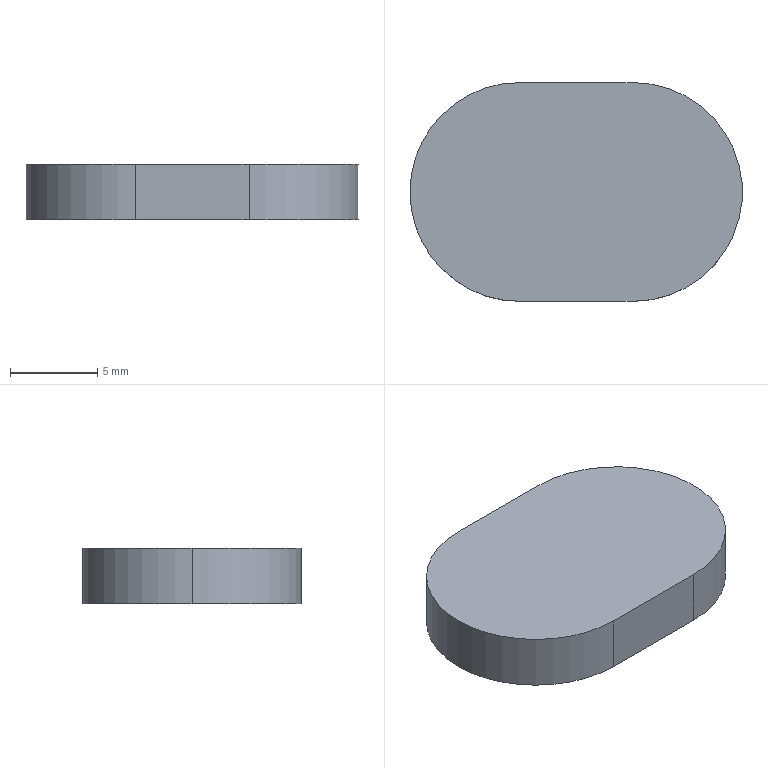Part | SolidWorks | features FlatPattern 1, SMBaseFlange 1, SheetMetal 1 | 1 solid | 7 faces | box 19 x 12.5 x 3.2 mm | volume 652.699 mm3 | plane 4 | cylinder 3 | commonest cylinder face diameters 12.5 x3
STEP:
#1=CARTESIAN_POINT('',(569.5,720.,3.2));
#2=VERTEX_POINT('',#1);
#3=CARTESIAN_POINT('',(575.75,713.75,3.2));
#4=VERTEX_POINT('',#3);
#5=CARTESIAN_POINT('',(575.75,720.,3.2));
#6=DIRECTION('',(0.,0.,1.));
#7=DIRECTION('',(1.,0.,0.));
#8=AXIS2_PLACEMENT_3D('',#5,#6,#7);
#9=CIRCLE('',#8,6.25);
#10=EDGE_CURVE('',#2,#4,#9,.T.);
#11=ORIENTED_EDGE('',*,*,#10,.F.);
#12=CARTESIAN_POINT('',(569.5,720.,0.));
#13=VERTEX_POINT('',#12);
#14=CARTESIAN_POINT('',(569.5,720.,3.2));
#15=DIRECTION('',(0.,0.,-1.));
#16=VECTOR('',#15,1000.);
#17=LINE('',#14,#16);
#18=EDGE_CURVE('',#2,#13,#17,.T.);
#19=ORIENTED_EDGE('',*,*,#18,.T.);
#20=CARTESIAN_POINT('',(575.75,713.75,0.));
#21=VERTEX_POINT('',#20);
#22=CARTESIAN_POINT('',(575.75,720.,0.));
#23=DIRECTION('',(0.,0.,1.));
#24=DIRECTION('',(1.,0.,0.));
#25=AXIS2_PLACEMENT_3D('',#22,#23,#24);
#26=CIRCLE('',#25,6.25);
#27=EDGE_CURVE('',#13,#21,#26,.T.);
#28=ORIENTED_EDGE('',*,*,#27,.T.);
#29=CARTESIAN_POINT('',(575.75,713.75,3.2));
#30=DIRECTION('',(0.,0.,-1.));
#31=VECTOR('',#30,1000.);
#32=LINE('',#29,#31);
#33=EDGE_CURVE('',#4,#21,#32,.T.);
#34=ORIENTED_EDGE('',*,*,#33,.F.);
#35=EDGE_LOOP('',(#11,#19,#28,#34));
#36=FACE_OUTER_BOUND('',#35,.T.);
#37=CARTESIAN_POINT('',(575.75,720.,3.2));
#38=DIRECTION('',(0.,0.,-1.));
#39=DIRECTION('',(-1.,0.,0.));
#40=AXIS2_PLACEMENT_3D('',#37,#38,#39);
#41=CYLINDRICAL_SURFACE('',#40,6.25);
#42=ADVANCED_FACE('',(#36),#41,.T.);
#43=ORIENTED_EDGE('',*,*,#18,.F.);
#44=CARTESIAN_POINT('',(575.75,726.25,3.2));
#45=VERTEX_POINT('',#44);
#46=CARTESIAN_POINT('',(575.75,720.,3.2));
#47=DIRECTION('',(0.,0.,1.));
#48=DIRECTION('',(1.,0.,0.));
#49=AXIS2_PLACEMENT_3D('',#46,#47,#48);
#50=CIRCLE('',#49,6.25);
#51=EDGE_CURVE('',#45,#2,#50,.T.);
#52=ORIENTED_EDGE('',*,*,#51,.F.);
#53=CARTESIAN_POINT('',(575.75,726.25,0.));
#54=VERTEX_POINT('',#53);
#55=CARTESIAN_POINT('',(575.75,726.25,3.2));
#56=DIRECTION('',(0.,0.,-1.));
#57=VECTOR('',#56,1000.);
#58=LINE('',#55,#57);
#59=EDGE_CURVE('',#45,#54,#58,.T.);
#60=ORIENTED_EDGE('',*,*,#59,.T.);
#61=CARTESIAN_POINT('',(575.75,720.,0.));
#62=DIRECTION('',(0.,0.,1.));
#63=DIRECTION('',(1.,0.,0.));
#64=AXIS2_PLACEMENT_3D('',#61,#62,#63);
#65=CIRCLE('',#64,6.25);
#66=EDGE_CURVE('',#54,#13,#65,.T.);
#67=ORIENTED_EDGE('',*,*,#66,.T.);
#68=EDGE_LOOP('',(#43,#52,#60,#67));
#69=FACE_OUTER_BOUND('',#68,.T.);
#70=CARTESIAN_POINT('',(575.75,720.,3.2));
#71=DIRECTION('',(0.,0.,-1.));
#72=DIRECTION('',(-1.,0.,0.));
#73=AXIS2_PLACEMENT_3D('',#70,#71,#72);
#74=CYLINDRICAL_SURFACE('',#73,6.25);
#75=ADVANCED_FACE('',(#69),#74,.T.);
#76=CARTESIAN_POINT('',(582.25,713.75,0.));
#77=VERTEX_POINT('',#76);
#78=CARTESIAN_POINT('',(575.75,713.75,0.));
#79=DIRECTION('',(1.,0.,0.));
#80=VECTOR('',#79,1000.);
#81=LINE('',#78,#80);
#82=EDGE_CURVE('',#21,#77,#81,.T.);
#83=ORIENTED_EDGE('',*,*,#82,.T.);
#84=CARTESIAN_POINT('',(582.25,713.75,3.2));
#85=VERTEX_POINT('',#84);
#86=CARTESIAN_POINT('',(582.25,713.75,3.2));
#87=DIRECTION('',(0.,0.,-1.));
#88=VECTOR('',#87,1000.);
#89=LINE('',#86,#88);
#90=EDGE_CURVE('',#85,#77,#89,.T.);
#91=ORIENTED_EDGE('',*,*,#90,.F.);
#92=CARTESIAN_POINT('',(575.75,713.75,3.2));
#93=DIRECTION('',(1.,0.,0.));
#94=VECTOR('',#93,1000.);
#95=LINE('',#92,#94);
#96=EDGE_CURVE('',#4,#85,#95,.T.);
#97=ORIENTED_EDGE('',*,*,#96,.F.);
#98=ORIENTED_EDGE('',*,*,#33,.T.);
#99=EDGE_LOOP('',(#83,#91,#97,#98));
#100=FACE_OUTER_BOUND('',#99,.T.);
#101=CARTESIAN_POINT('',(575.75,713.75,3.2));
#102=DIRECTION('',(0.,1.,0.));
#103=DIRECTION('',(0.,0.,1.));
#104=AXIS2_PLACEMENT_3D('',#101,#102,#103);
#105=PLANE('',#104);
#106=ADVANCED_FACE('',(#100),#105,.F.);
#107=CARTESIAN_POINT('',(582.25,726.25,0.));
#108=VERTEX_POINT('',#107);
#109=CARTESIAN_POINT('',(582.25,720.,0.));
#110=DIRECTION('',(0.,0.,1.));
#111=DIRECTION('',(1.,0.,0.));
#112=AXIS2_PLACEMENT_3D('',#109,#110,#111);
#113=CIRCLE('',#112,6.25);
#114=EDGE_CURVE('',#77,#108,#113,.T.);
#115=ORIENTED_EDGE('',*,*,#114,.T.);
#116=CARTESIAN_POINT('',(582.25,726.25,3.2));
#117=VERTEX_POINT('',#116);
#118=CARTESIAN_POINT('',(582.25,726.25,3.2));
#119=DIRECTION('',(0.,0.,-1.));
#120=VECTOR('',#119,1000.);
#121=LINE('',#118,#120);
#122=EDGE_CURVE('',#117,#108,#121,.T.);
#123=ORIENTED_EDGE('',*,*,#122,.F.);
#124=CARTESIAN_POINT('',(582.25,720.,3.2));
#125=DIRECTION('',(0.,0.,1.));
#126=DIRECTION('',(1.,0.,0.));
#127=AXIS2_PLACEMENT_3D('',#124,#125,#126);
#128=CIRCLE('',#127,6.25);
#129=EDGE_CURVE('',#85,#117,#128,.T.);
#130=ORIENTED_EDGE('',*,*,#129,.F.);
#131=ORIENTED_EDGE('',*,*,#90,.T.);
#132=EDGE_LOOP('',(#115,#123,#130,#131));
#133=FACE_OUTER_BOUND('',#132,.T.);
#134=CARTESIAN_POINT('',(582.25,720.,3.2));
#135=DIRECTION('',(0.,0.,-1.));
#136=DIRECTION('',(-1.,0.,0.));
#137=AXIS2_PLACEMENT_3D('',#134,#135,#136);
#138=CYLINDRICAL_SURFACE('',#137,6.25);
#139=ADVANCED_FACE('',(#133),#138,.T.);
#140=CARTESIAN_POINT('',(575.75,726.25,0.));
#141=DIRECTION('',(-1.,0.,0.));
#142=VECTOR('',#141,1000.);
#143=LINE('',#140,#142);
#144=EDGE_CURVE('',#108,#54,#143,.T.);
#145=ORIENTED_EDGE('',*,*,#144,.T.);
#146=ORIENTED_EDGE('',*,*,#59,.F.);
#147=CARTESIAN_POINT('',(575.75,726.25,3.2));
#148=DIRECTION('',(-1.,0.,0.));
#149=VECTOR('',#148,1000.);
#150=LINE('',#147,#149);
#151=EDGE_CURVE('',#117,#45,#150,.T.);
#152=ORIENTED_EDGE('',*,*,#151,.F.);
#153=ORIENTED_EDGE('',*,*,#122,.T.);
#154=EDGE_LOOP('',(#145,#146,#152,#153));
#155=FACE_OUTER_BOUND('',#154,.T.);
#156=CARTESIAN_POINT('',(575.75,726.25,3.2));
#157=DIRECTION('',(0.,-1.,0.));
#158=DIRECTION('',(0.,0.,-1.));
#159=AXIS2_PLACEMENT_3D('',#156,#157,#158);
#160=PLANE('',#159);
#161=ADVANCED_FACE('',(#155),#160,.F.);
#162=ORIENTED_EDGE('',*,*,#51,.T.);
#163=ORIENTED_EDGE('',*,*,#10,.T.);
#164=ORIENTED_EDGE('',*,*,#96,.T.);
#165=ORIENTED_EDGE('',*,*,#129,.T.);
#166=ORIENTED_EDGE('',*,*,#151,.T.);
#167=EDGE_LOOP('',(#162,#163,#164,#165,#166));
#168=FACE_OUTER_BOUND('',#167,.T.);
#169=CARTESIAN_POINT('',(575.75,720.,3.2));
#170=DIRECTION('',(0.,0.,1.));
#171=DIRECTION('',(1.,0.,0.));
#172=AXIS2_PLACEMENT_3D('',#169,#170,#171);
#173=PLANE('',#172);
#174=ADVANCED_FACE('',(#168),#173,.T.);
#175=ORIENTED_EDGE('',*,*,#66,.F.);
#176=ORIENTED_EDGE('',*,*,#144,.F.);
#177=ORIENTED_EDGE('',*,*,#114,.F.);
#178=ORIENTED_EDGE('',*,*,#82,.F.);
#179=ORIENTED_EDGE('',*,*,#27,.F.);
#180=EDGE_LOOP('',(#175,#176,#177,#178,#179));
#181=FACE_OUTER_BOUND('',#180,.T.);
#182=CARTESIAN_POINT('',(575.75,720.,0.));
#183=DIRECTION('',(0.,0.,1.));
#184=DIRECTION('',(1.,0.,0.));
#185=AXIS2_PLACEMENT_3D('',#182,#183,#184);
#186=PLANE('',#185);
#187=ADVANCED_FACE('',(#181),#186,.F.);
#188=CLOSED_SHELL('',(#42,#75,#106,#139,#161,#174,#187));
#189=MANIFOLD_SOLID_BREP('',#188);
#190=CARTESIAN_POINT('',(0.,0.,0.));
#191=DIRECTION('',(0.,0.,1.));
#192=DIRECTION('',(1.,0.,0.));
#193=AXIS2_PLACEMENT_3D('',#190,#191,#192);
#194=(LENGTH_UNIT()NAMED_UNIT(*)SI_UNIT(.MILLI.,.METRE.));
#195=UNCERTAINTY_MEASURE_WITH_UNIT(LENGTH_MEASURE(0.00001),#194,'','');
#196=(NAMED_UNIT(*)PLANE_ANGLE_UNIT()SI_UNIT($,.RADIAN.));
#197=(NAMED_UNIT(*)SI_UNIT($,.STERADIAN.)SOLID_ANGLE_UNIT());
#198=(GEOMETRIC_REPRESENTATION_CONTEXT(3)GLOBAL_UNCERTAINTY_ASSIGNED_CONTEXT((#195))GLOBAL_UNIT_ASSIGNED_CONTEXT((#194,#196,#197))REPRESENTATION_CONTEXT('',''));
#199=ADVANCED_BREP_SHAPE_REPRESENTATION('',(#189,#193),#198);